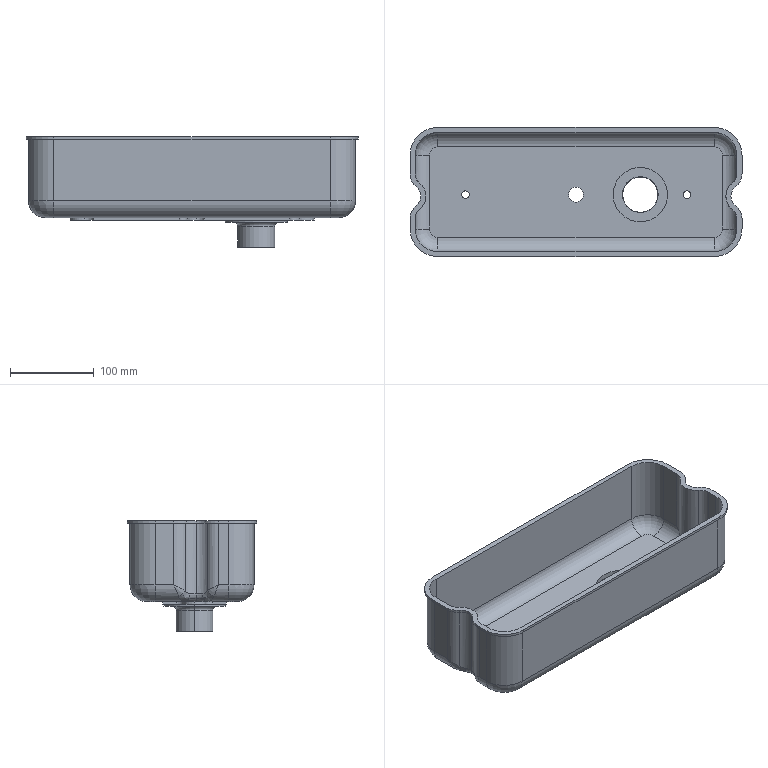Part | SolidWorks | features BaseBody 2 | 2 solids | 139 faces | box 396 x 154 x 132 mm | volume 484114 mm3 | cylinder 77 | plane 41 | torus 13 | spline 8 | commonest cylinder face diameters 40 x13 34 x11 18 x10 28 x7 14 x5 27 x5